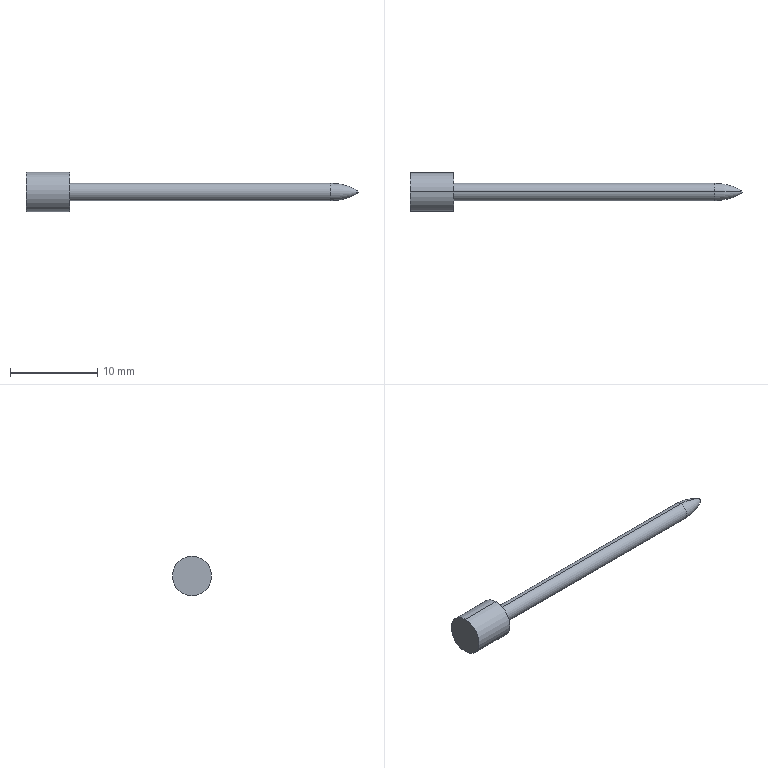Part | STEP file | BU-A09 | 1 solid | 10 faces | box 38.05 x 4.5 x 4.5 mm | volume 179.303 mm3 | cylinder 4 | plane 2 | other 2 | sphere 2 | commonest cylinder face diameters 2 x2 4.5 x2
STEP:
#1=CARTESIAN_POINT('',(0.,0.,0.));
#2=DIRECTION('',(0.,0.,1.));
#3=DIRECTION('',(1.,0.,0.));
#4=AXIS2_PLACEMENT_3D('',#1,#2,#3);
#5=CARTESIAN_POINT('',(5.,0.,2.25));
#6=VERTEX_POINT('',#5);
#7=CARTESIAN_POINT('',(5.,0.,-2.25));
#8=VERTEX_POINT('',#7);
#9=CARTESIAN_POINT('',(5.,0.,0.));
#10=DIRECTION('',(-1.,0.,0.));
#11=DIRECTION('',(0.,0.,1.));
#12=AXIS2_PLACEMENT_3D('',#9,#10,#11);
#13=CIRCLE('',#12,2.25);
#14=CARTESIAN_POINT('',(-1000.,0.,0.));
#15=DIRECTION('',(-1.,0.,0.));
#16=DIRECTION('',(0.,0.,1.));
#17=AXIS2_PLACEMENT_3D('',#14,#15,#16);
#18=CYLINDRICAL_SURFACE('',#17,2.25);
#19=CARTESIAN_POINT('',(0.,-1005.));
#20=DIRECTION('',(1.,0.));
#21=VECTOR('',#20,1.);
#22=LINE('',#19,#21);
#23=(GEOMETRIC_REPRESENTATION_CONTEXT(2)PARAMETRIC_REPRESENTATION_CONTEXT()REPRESENTATION_CONTEXT('',''));
#24=DEFINITIONAL_REPRESENTATION('',(#22),#23);
#25=PCURVE('',#18,#24);
#26=CARTESIAN_POINT('',(5.,2.25,0.));
#27=DIRECTION('',(-1.,0.,0.));
#28=DIRECTION('',(0.,0.,1.));
#29=AXIS2_PLACEMENT_3D('',#26,#27,#28);
#30=PLANE('',#29);
#31=CARTESIAN_POINT('',(0.,-2.25));
#32=DIRECTION('',(1.,0.));
#33=AXIS2_PLACEMENT_2D('',#31,#32);
#34=CIRCLE('',#33,2.25);
#35=(GEOMETRIC_REPRESENTATION_CONTEXT(2)PARAMETRIC_REPRESENTATION_CONTEXT()REPRESENTATION_CONTEXT('',''));
#36=DEFINITIONAL_REPRESENTATION('',(#34),#35);
#37=PCURVE('',#30,#36);
#38=SURFACE_CURVE('',#13,(#25,#37),.PCURVE_S1.);
#39=EDGE_CURVE('',#6,#8,#38,.T.);
#40=ORIENTED_EDGE('',*,*,#39,.T.);
#41=CARTESIAN_POINT('',(0.,0.,-2.25));
#42=VERTEX_POINT('',#41);
#43=CARTESIAN_POINT('',(-1000.,0.,-2.25));
#44=DIRECTION('',(-1.,0.,0.));
#45=VECTOR('',#44,1.);
#46=LINE('',#43,#45);
#47=CARTESIAN_POINT('',(3.142,0.));
#48=DIRECTION('',(0.,1.));
#49=VECTOR('',#48,1.);
#50=LINE('',#47,#49);
#51=(GEOMETRIC_REPRESENTATION_CONTEXT(2)PARAMETRIC_REPRESENTATION_CONTEXT()REPRESENTATION_CONTEXT('',''));
#52=DEFINITIONAL_REPRESENTATION('',(#50),#51);
#53=PCURVE('',#18,#52);
#54=CARTESIAN_POINT('',(-1000.,0.,0.));
#55=DIRECTION('',(-1.,0.,0.));
#56=DIRECTION('',(0.,0.,1.));
#57=AXIS2_PLACEMENT_3D('',#54,#55,#56);
#58=CYLINDRICAL_SURFACE('',#57,2.25);
#59=CARTESIAN_POINT('',(3.142,0.));
#60=DIRECTION('',(0.,1.));
#61=VECTOR('',#60,1.);
#62=LINE('',#59,#61);
#63=(GEOMETRIC_REPRESENTATION_CONTEXT(2)PARAMETRIC_REPRESENTATION_CONTEXT()REPRESENTATION_CONTEXT('',''));
#64=DEFINITIONAL_REPRESENTATION('',(#62),#63);
#65=PCURVE('',#58,#64);
#66=SURFACE_CURVE('',#46,(#53,#65),.PCURVE_S1.);
#67=EDGE_CURVE('',#8,#42,#66,.T.);
#68=ORIENTED_EDGE('',*,*,#67,.T.);
#69=CARTESIAN_POINT('',(0.,0.,2.25));
#70=VERTEX_POINT('',#69);
#71=CARTESIAN_POINT('',(0.,0.,0.));
#72=DIRECTION('',(-1.,0.,0.));
#73=DIRECTION('',(0.,0.,1.));
#74=AXIS2_PLACEMENT_3D('',#71,#72,#73);
#75=CIRCLE('',#74,2.25);
#76=CARTESIAN_POINT('',(0.,-1000.));
#77=DIRECTION('',(1.,0.));
#78=VECTOR('',#77,1.);
#79=LINE('',#76,#78);
#80=(GEOMETRIC_REPRESENTATION_CONTEXT(2)PARAMETRIC_REPRESENTATION_CONTEXT()REPRESENTATION_CONTEXT('',''));
#81=DEFINITIONAL_REPRESENTATION('',(#79),#80);
#82=PCURVE('',#18,#81);
#83=CARTESIAN_POINT('',(0.,0.,0.));
#84=DIRECTION('',(1.,0.,0.));
#85=DIRECTION('',(0.,0.,-1.));
#86=AXIS2_PLACEMENT_3D('',#83,#84,#85);
#87=PLANE('',#86);
#88=CARTESIAN_POINT('',(-2.25,0.));
#89=CARTESIAN_POINT('',(-2.25,3.897));
#90=CARTESIAN_POINT('',(1.125,1.949));
#91=CARTESIAN_POINT('',(4.5,0.));
#92=CARTESIAN_POINT('',(1.125,-1.949));
#93=CARTESIAN_POINT('',(-2.25,-3.897));
#94=CARTESIAN_POINT('',(-2.25,0.));
#95=(BOUNDED_CURVE()B_SPLINE_CURVE(2,(#88,#89,#90,#91,#92,#93,#94),.UNSPECIFIED.,.T.,.F.)B_SPLINE_CURVE_WITH_KNOTS((1,2,2,2,2,1),(-2.094,0.,2.094,4.189,6.283,8.378),.UNSPECIFIED.)CURVE()GEOMETRIC_REPRESENTATION_ITEM()RATIONAL_B_SPLINE_CURVE((1.,0.5,1.,0.5,1.,0.5,1.))REPRESENTATION_ITEM(''));
#96=(GEOMETRIC_REPRESENTATION_CONTEXT(2)PARAMETRIC_REPRESENTATION_CONTEXT()REPRESENTATION_CONTEXT('',''));
#97=DEFINITIONAL_REPRESENTATION('',(#95),#96);
#98=PCURVE('',#87,#97);
#99=SURFACE_CURVE('',#75,(#82,#98),.PCURVE_S1.);
#100=EDGE_CURVE('',#70,#42,#99,.T.);
#101=ORIENTED_EDGE('',*,*,#100,.F.);
#102=CARTESIAN_POINT('',(-1000.,0.,2.25));
#103=DIRECTION('',(-1.,0.,0.));
#104=VECTOR('',#103,1.);
#105=LINE('',#102,#104);
#106=CARTESIAN_POINT('',(0.,0.));
#107=DIRECTION('',(0.,1.));
#108=VECTOR('',#107,1.);
#109=LINE('',#106,#108);
#110=(GEOMETRIC_REPRESENTATION_CONTEXT(2)PARAMETRIC_REPRESENTATION_CONTEXT()REPRESENTATION_CONTEXT('',''));
#111=DEFINITIONAL_REPRESENTATION('',(#109),#110);
#112=PCURVE('',#18,#111);
#113=CARTESIAN_POINT('',(6.283,0.));
#114=DIRECTION('',(0.,1.));
#115=VECTOR('',#114,1.);
#116=LINE('',#113,#115);
#117=(GEOMETRIC_REPRESENTATION_CONTEXT(2)PARAMETRIC_REPRESENTATION_CONTEXT()REPRESENTATION_CONTEXT('',''));
#118=DEFINITIONAL_REPRESENTATION('',(#116),#117);
#119=PCURVE('',#58,#118);
#120=SURFACE_CURVE('',#105,(#112,#119),.PCURVE_S1.);
#121=EDGE_CURVE('',#6,#70,#120,.T.);
#122=ORIENTED_EDGE('',*,*,#121,.F.);
#123=EDGE_LOOP('',(#40,#68,#101,#122));
#124=FACE_BOUND('',#123,.T.);
#125=ADVANCED_FACE('',(#124),#18,.T.);
#126=ORIENTED_EDGE('',*,*,#100,.T.);
#127=CARTESIAN_POINT('',(0.,0.,0.));
#128=DIRECTION('',(-1.,0.,0.));
#129=DIRECTION('',(0.,0.,1.));
#130=AXIS2_PLACEMENT_3D('',#127,#128,#129);
#131=CIRCLE('',#130,2.25);
#132=CARTESIAN_POINT('',(-2.25,0.));
#133=CARTESIAN_POINT('',(-2.25,3.897));
#134=CARTESIAN_POINT('',(1.125,1.949));
#135=CARTESIAN_POINT('',(4.5,0.));
#136=CARTESIAN_POINT('',(1.125,-1.949));
#137=CARTESIAN_POINT('',(-2.25,-3.897));
#138=CARTESIAN_POINT('',(-2.25,0.));
#139=(BOUNDED_CURVE()B_SPLINE_CURVE(2,(#132,#133,#134,#135,#136,#137,#138),.UNSPECIFIED.,.T.,.F.)B_SPLINE_CURVE_WITH_KNOTS((1,2,2,2,2,1),(-2.094,0.,2.094,4.189,6.283,8.378),.UNSPECIFIED.)CURVE()GEOMETRIC_REPRESENTATION_ITEM()RATIONAL_B_SPLINE_CURVE((1.,0.5,1.,0.5,1.,0.5,1.))REPRESENTATION_ITEM(''));
#140=(GEOMETRIC_REPRESENTATION_CONTEXT(2)PARAMETRIC_REPRESENTATION_CONTEXT()REPRESENTATION_CONTEXT('',''));
#141=DEFINITIONAL_REPRESENTATION('',(#139),#140);
#142=PCURVE('',#87,#141);
#143=CARTESIAN_POINT('',(0.,-1000.));
#144=DIRECTION('',(1.,0.));
#145=VECTOR('',#144,1.);
#146=LINE('',#143,#145);
#147=(GEOMETRIC_REPRESENTATION_CONTEXT(2)PARAMETRIC_REPRESENTATION_CONTEXT()REPRESENTATION_CONTEXT('',''));
#148=DEFINITIONAL_REPRESENTATION('',(#146),#147);
#149=PCURVE('',#58,#148);
#150=SURFACE_CURVE('',#131,(#142,#149),.PCURVE_S1.);
#151=EDGE_CURVE('',#42,#70,#150,.T.);
#152=ORIENTED_EDGE('',*,*,#151,.T.);
#153=EDGE_LOOP('',(#126,#152));
#154=FACE_BOUND('',#153,.T.);
#155=ADVANCED_FACE('',(#154),#87,.F.);
#156=ORIENTED_EDGE('',*,*,#67,.F.);
#157=CARTESIAN_POINT('',(5.,0.,0.));
#158=DIRECTION('',(-1.,0.,0.));
#159=DIRECTION('',(0.,0.,1.));
#160=AXIS2_PLACEMENT_3D('',#157,#158,#159);
#161=CIRCLE('',#160,2.25);
#162=CARTESIAN_POINT('',(0.,-1005.));
#163=DIRECTION('',(1.,0.));
#164=VECTOR('',#163,1.);
#165=LINE('',#162,#164);
#166=(GEOMETRIC_REPRESENTATION_CONTEXT(2)PARAMETRIC_REPRESENTATION_CONTEXT()REPRESENTATION_CONTEXT('',''));
#167=DEFINITIONAL_REPRESENTATION('',(#165),#166);
#168=PCURVE('',#58,#167);
#169=CARTESIAN_POINT('',(0.,-2.25));
#170=DIRECTION('',(1.,0.));
#171=AXIS2_PLACEMENT_2D('',#169,#170);
#172=CIRCLE('',#171,2.25);
#173=(GEOMETRIC_REPRESENTATION_CONTEXT(2)PARAMETRIC_REPRESENTATION_CONTEXT()REPRESENTATION_CONTEXT('',''));
#174=DEFINITIONAL_REPRESENTATION('',(#172),#173);
#175=PCURVE('',#30,#174);
#176=SURFACE_CURVE('',#161,(#168,#175),.PCURVE_S1.);
#177=EDGE_CURVE('',#8,#6,#176,.T.);
#178=ORIENTED_EDGE('',*,*,#177,.T.);
#179=ORIENTED_EDGE('',*,*,#121,.T.);
#180=ORIENTED_EDGE('',*,*,#151,.F.);
#181=EDGE_LOOP('',(#156,#178,#179,#180));
#182=FACE_BOUND('',#181,.T.);
#183=ADVANCED_FACE('',(#182),#58,.T.);
#184=ORIENTED_EDGE('',*,*,#39,.F.);
#185=ORIENTED_EDGE('',*,*,#177,.F.);
#186=EDGE_LOOP('',(#184,#185));
#187=FACE_BOUND('',#186,.T.);
#188=CARTESIAN_POINT('',(5.,0.,1.));
#189=VERTEX_POINT('',#188);
#190=CARTESIAN_POINT('',(5.,0.,-1.));
#191=VERTEX_POINT('',#190);
#192=CARTESIAN_POINT('',(5.,0.,0.));
#193=DIRECTION('',(-1.,0.,0.));
#194=DIRECTION('',(0.,0.,1.));
#195=AXIS2_PLACEMENT_3D('',#192,#193,#194);
#196=CIRCLE('',#195,1.);
#197=CARTESIAN_POINT('',(0.,-2.25));
#198=DIRECTION('',(1.,0.));
#199=AXIS2_PLACEMENT_2D('',#197,#198);
#200=CIRCLE('',#199,1.);
#201=(GEOMETRIC_REPRESENTATION_CONTEXT(2)PARAMETRIC_REPRESENTATION_CONTEXT()REPRESENTATION_CONTEXT('',''));
#202=DEFINITIONAL_REPRESENTATION('',(#200),#201);
#203=PCURVE('',#30,#202);
#204=CARTESIAN_POINT('',(-1000.,0.,0.));
#205=DIRECTION('',(-1.,0.,0.));
#206=DIRECTION('',(0.,0.,1.));
#207=AXIS2_PLACEMENT_3D('',#204,#205,#206);
#208=CYLINDRICAL_SURFACE('',#207,1.);
#209=CARTESIAN_POINT('',(0.,-1005.));
#210=DIRECTION('',(1.,0.));
#211=VECTOR('',#210,1.);
#212=LINE('',#209,#211);
#213=(GEOMETRIC_REPRESENTATION_CONTEXT(2)PARAMETRIC_REPRESENTATION_CONTEXT()REPRESENTATION_CONTEXT('',''));
#214=DEFINITIONAL_REPRESENTATION('',(#212),#213);
#215=PCURVE('',#208,#214);
#216=SURFACE_CURVE('',#196,(#203,#215),.PCURVE_S1.);
#217=EDGE_CURVE('',#189,#191,#216,.T.);
#218=ORIENTED_EDGE('',*,*,#217,.T.);
#219=CARTESIAN_POINT('',(5.,0.,0.));
#220=DIRECTION('',(-1.,0.,0.));
#221=DIRECTION('',(0.,0.,1.));
#222=AXIS2_PLACEMENT_3D('',#219,#220,#221);
#223=CIRCLE('',#222,1.);
#224=CARTESIAN_POINT('',(0.,-2.25));
#225=DIRECTION('',(1.,0.));
#226=AXIS2_PLACEMENT_2D('',#224,#225);
#227=CIRCLE('',#226,1.);
#228=(GEOMETRIC_REPRESENTATION_CONTEXT(2)PARAMETRIC_REPRESENTATION_CONTEXT()REPRESENTATION_CONTEXT('',''));
#229=DEFINITIONAL_REPRESENTATION('',(#227),#228);
#230=PCURVE('',#30,#229);
#231=CARTESIAN_POINT('',(-1000.,0.,0.));
#232=DIRECTION('',(-1.,0.,0.));
#233=DIRECTION('',(0.,0.,1.));
#234=AXIS2_PLACEMENT_3D('',#231,#232,#233);
#235=CYLINDRICAL_SURFACE('',#234,1.);
#236=CARTESIAN_POINT('',(0.,-1005.));
#237=DIRECTION('',(1.,0.));
#238=VECTOR('',#237,1.);
#239=LINE('',#236,#238);
#240=(GEOMETRIC_REPRESENTATION_CONTEXT(2)PARAMETRIC_REPRESENTATION_CONTEXT()REPRESENTATION_CONTEXT('',''));
#241=DEFINITIONAL_REPRESENTATION('',(#239),#240);
#242=PCURVE('',#235,#241);
#243=SURFACE_CURVE('',#223,(#230,#242),.PCURVE_S1.);
#244=EDGE_CURVE('',#191,#189,#243,.T.);
#245=ORIENTED_EDGE('',*,*,#244,.T.);
#246=EDGE_LOOP('',(#218,#245));
#247=FACE_BOUND('',#246,.T.);
#248=ADVANCED_FACE('',(#187,#247),#30,.F.);
#249=CARTESIAN_POINT('',(34.934,0.,-1.));
#250=VERTEX_POINT('',#249);
#251=CARTESIAN_POINT('',(-1000.,0.,-1.));
#252=DIRECTION('',(-1.,0.,0.));
#253=VECTOR('',#252,1.);
#254=LINE('',#251,#253);
#255=CARTESIAN_POINT('',(3.142,0.));
#256=DIRECTION('',(0.,1.));
#257=VECTOR('',#256,1.);
#258=LINE('',#255,#257);
#259=(GEOMETRIC_REPRESENTATION_CONTEXT(2)PARAMETRIC_REPRESENTATION_CONTEXT()REPRESENTATION_CONTEXT('',''));
#260=DEFINITIONAL_REPRESENTATION('',(#258),#259);
#261=PCURVE('',#235,#260);
#262=CARTESIAN_POINT('',(3.142,0.));
#263=DIRECTION('',(0.,1.));
#264=VECTOR('',#263,1.);
#265=LINE('',#262,#264);
#266=(GEOMETRIC_REPRESENTATION_CONTEXT(2)PARAMETRIC_REPRESENTATION_CONTEXT()REPRESENTATION_CONTEXT('',''));
#267=DEFINITIONAL_REPRESENTATION('',(#265),#266);
#268=PCURVE('',#208,#267);
#269=SURFACE_CURVE('',#254,(#261,#268),.PCURVE_S1.);
#270=EDGE_CURVE('',#250,#191,#269,.T.);
#271=ORIENTED_EDGE('',*,*,#270,.F.);
#272=CARTESIAN_POINT('',(34.934,0.,1.));
#273=VERTEX_POINT('',#272);
#274=CARTESIAN_POINT('',(34.934,0.,0.));
#275=DIRECTION('',(-1.,0.,0.));
#276=DIRECTION('',(0.,0.,1.));
#277=AXIS2_PLACEMENT_3D('',#274,#275,#276);
#278=CIRCLE('',#277,1.);
#279=CARTESIAN_POINT('',(0.,-1034.934));
#280=DIRECTION('',(1.,0.));
#281=VECTOR('',#280,1.);
#282=LINE('',#279,#281);
#283=(GEOMETRIC_REPRESENTATION_CONTEXT(2)PARAMETRIC_REPRESENTATION_CONTEXT()REPRESENTATION_CONTEXT('',''));
#284=DEFINITIONAL_REPRESENTATION('',(#282),#283);
#285=PCURVE('',#235,#284);
#286=CARTESIAN_POINT('',(34.934,0.,-1.));
#287=CARTESIAN_POINT('',(35.559,0.,-1.));
#288=CARTESIAN_POINT('',(36.183,0.,-0.9201));
#289=CARTESIAN_POINT('',(36.794,0.,-0.7602));
#290=CARTESIAN_POINT('',(37.378,0.,-0.5239));
#291=CARTESIAN_POINT('',(37.922,0.,-0.2179));
#292=B_SPLINE_CURVE_WITH_KNOTS('',5,(#286,#287,#288,#289,#290,#291),.UNSPECIFIED.,.F.,.F.,(6,6),(3.142,3.654),.PIECEWISE_BEZIER_KNOTS.);
#293=CARTESIAN_POINT('',(34.934,0.,0.));
#294=DIRECTION('',(-1.,0.,0.));
#295=AXIS1_PLACEMENT('',#293,#294);
#296=SURFACE_OF_REVOLUTION('',#292,#295);
#297=CARTESIAN_POINT('',(-3.142,3.142));
#298=DIRECTION('',(1.,0.));
#299=VECTOR('',#298,1.);
#300=LINE('',#297,#299);
#301=(GEOMETRIC_REPRESENTATION_CONTEXT(2)PARAMETRIC_REPRESENTATION_CONTEXT()REPRESENTATION_CONTEXT('',''));
#302=DEFINITIONAL_REPRESENTATION('',(#300),#301);
#303=PCURVE('',#296,#302);
#304=SURFACE_CURVE('',#278,(#285,#303),.PCURVE_S1.);
#305=EDGE_CURVE('',#250,#273,#304,.T.);
#306=ORIENTED_EDGE('',*,*,#305,.T.);
#307=CARTESIAN_POINT('',(-1000.,0.,1.));
#308=DIRECTION('',(-1.,0.,0.));
#309=VECTOR('',#308,1.);
#310=LINE('',#307,#309);
#311=CARTESIAN_POINT('',(6.283,0.));
#312=DIRECTION('',(0.,1.));
#313=VECTOR('',#312,1.);
#314=LINE('',#311,#313);
#315=(GEOMETRIC_REPRESENTATION_CONTEXT(2)PARAMETRIC_REPRESENTATION_CONTEXT()REPRESENTATION_CONTEXT('',''));
#316=DEFINITIONAL_REPRESENTATION('',(#314),#315);
#317=PCURVE('',#235,#316);
#318=CARTESIAN_POINT('',(0.,0.));
#319=DIRECTION('',(0.,1.));
#320=VECTOR('',#319,1.);
#321=LINE('',#318,#320);
#322=(GEOMETRIC_REPRESENTATION_CONTEXT(2)PARAMETRIC_REPRESENTATION_CONTEXT()REPRESENTATION_CONTEXT('',''));
#323=DEFINITIONAL_REPRESENTATION('',(#321),#322);
#324=PCURVE('',#208,#323);
#325=SURFACE_CURVE('',#310,(#317,#324),.PCURVE_S1.);
#326=EDGE_CURVE('',#273,#189,#325,.T.);
#327=ORIENTED_EDGE('',*,*,#326,.T.);
#328=ORIENTED_EDGE('',*,*,#244,.F.);
#329=EDGE_LOOP('',(#271,#306,#327,#328));
#330=FACE_BOUND('',#329,.T.);
#331=ADVANCED_FACE('',(#330),#235,.T.);
#332=ORIENTED_EDGE('',*,*,#305,.T.);
#333=CARTESIAN_POINT('',(37.922,0.,0.2179));
#334=VERTEX_POINT('',#333);
#335=CARTESIAN_POINT('',(34.934,0.,-5.1));
#336=DIRECTION('',(0.,-1.,0.));
#337=DIRECTION('',(1.,0.,0.));
#338=AXIS2_PLACEMENT_3D('',#335,#336,#337);
#339=CIRCLE('',#338,6.1);
#340=CARTESIAN_POINT('',(3.142,4.712));
#341=DIRECTION('',(0.,-1.));
#342=VECTOR('',#341,1.);
#343=LINE('',#340,#342);
#344=(GEOMETRIC_REPRESENTATION_CONTEXT(2)PARAMETRIC_REPRESENTATION_CONTEXT()REPRESENTATION_CONTEXT('',''));
#345=DEFINITIONAL_REPRESENTATION('',(#343),#344);
#346=PCURVE('',#296,#345);
#347=CARTESIAN_POINT('',(34.934,0.,-1.));
#348=CARTESIAN_POINT('',(35.559,0.,-1.));
#349=CARTESIAN_POINT('',(36.183,0.,-0.9201));
#350=CARTESIAN_POINT('',(36.794,0.,-0.7602));
#351=CARTESIAN_POINT('',(37.378,0.,-0.5239));
#352=CARTESIAN_POINT('',(37.922,0.,-0.2179));
#353=B_SPLINE_CURVE_WITH_KNOTS('',5,(#347,#348,#349,#350,#351,#352),.UNSPECIFIED.,.F.,.F.,(6,6),(3.142,3.654),.PIECEWISE_BEZIER_KNOTS.);
#354=CARTESIAN_POINT('',(34.934,0.,0.));
#355=DIRECTION('',(-1.,0.,0.));
#356=AXIS1_PLACEMENT('',#354,#355);
#357=SURFACE_OF_REVOLUTION('',#353,#356);
#358=CARTESIAN_POINT('',(3.142,4.712));
#359=DIRECTION('',(0.,-1.));
#360=VECTOR('',#359,1.);
#361=LINE('',#358,#360);
#362=(GEOMETRIC_REPRESENTATION_CONTEXT(2)PARAMETRIC_REPRESENTATION_CONTEXT()REPRESENTATION_CONTEXT('',''));
#363=DEFINITIONAL_REPRESENTATION('',(#361),#362);
#364=PCURVE('',#357,#363);
#365=SURFACE_CURVE('',#339,(#346,#364),.PCURVE_S1.);
#366=EDGE_CURVE('',#334,#273,#365,.T.);
#367=ORIENTED_EDGE('',*,*,#366,.F.);
#368=CARTESIAN_POINT('',(37.922,-0.2179,0.));
#369=VERTEX_POINT('',#368);
#370=CARTESIAN_POINT('',(37.922,0.,0.));
#371=DIRECTION('',(-1.,0.,0.));
#372=DIRECTION('',(0.,0.,1.));
#373=AXIS2_PLACEMENT_3D('',#370,#371,#372);
#374=CIRCLE('',#373,0.2179);
#375=CARTESIAN_POINT('',(-3.142,3.654));
#376=DIRECTION('',(1.,0.));
#377=VECTOR('',#376,1.);
#378=LINE('',#375,#377);
#379=(GEOMETRIC_REPRESENTATION_CONTEXT(2)PARAMETRIC_REPRESENTATION_CONTEXT()REPRESENTATION_CONTEXT('',''));
#380=DEFINITIONAL_REPRESENTATION('',(#378),#379);
#381=PCURVE('',#296,#380);
#382=CARTESIAN_POINT('',(37.8,0.,0.));
#383=DIRECTION('',(0.,0.,-1.));
#384=DIRECTION('',(0.,1.,0.));
#385=AXIS2_PLACEMENT_3D('',#382,#383,#384);
#386=SPHERICAL_SURFACE('',#385,0.25);
#387=CARTESIAN_POINT('',(2.63,0.));
#388=CARTESIAN_POINT('',(2.63,-0.02075));
#389=CARTESIAN_POINT('',(2.629,-0.06225));
#390=CARTESIAN_POINT('',(2.626,-0.1244));
#391=CARTESIAN_POINT('',(2.62,-0.1864));
#392=CARTESIAN_POINT('',(2.612,-0.2482));
#393=CARTESIAN_POINT('',(2.602,-0.3097));
#394=CARTESIAN_POINT('',(2.589,-0.3707));
#395=CARTESIAN_POINT('',(2.573,-0.4311));
#396=CARTESIAN_POINT('',(2.553,-0.4909));
#397=CARTESIAN_POINT('',(2.53,-0.5499));
#398=CARTESIAN_POINT('',(2.503,-0.6078));
#399=CARTESIAN_POINT('',(2.471,-0.6645));
#400=CARTESIAN_POINT('',(2.433,-0.7196));
#401=CARTESIAN_POINT('',(2.39,-0.7729));
#402=CARTESIAN_POINT('',(2.338,-0.8238));
#403=CARTESIAN_POINT('',(2.279,-0.8719));
#404=CARTESIAN_POINT('',(2.209,-0.9165));
#405=CARTESIAN_POINT('',(2.129,-0.9568));
#406=CARTESIAN_POINT('',(2.037,-0.9919));
#407=CARTESIAN_POINT('',(1.934,-1.021));
#408=CARTESIAN_POINT('',(1.82,-1.042));
#409=CARTESIAN_POINT('',(1.698,-1.056));
#410=CARTESIAN_POINT('',(1.613,-1.059));
#411=CARTESIAN_POINT('',(1.571,-1.059));
#412=B_SPLINE_CURVE_WITH_KNOTS('',3,(#387,#388,#389,#390,#391,#392,#393,#394,#395,#396,#397,#398,#399,#400,#401,#402,#403,#404,#405,#406,#407,#408,#409,#410,#411),.UNSPECIFIED.,.F.,.F.,(4,1,1,1,1,1,1,1,1,1,1,1,1,1,1,1,1,1,1,1,1,1,4),(4.712,4.784,4.855,4.927,4.998,5.069,5.141,5.212,5.284,5.355,5.426,5.498,5.569,5.641,5.712,5.783,5.855,5.926,5.998,6.069,6.14,6.212,6.283),.QUASI_UNIFORM_KNOTS.);
#413=(GEOMETRIC_REPRESENTATION_CONTEXT(2)PARAMETRIC_REPRESENTATION_CONTEXT()REPRESENTATION_CONTEXT('',''));
#414=DEFINITIONAL_REPRESENTATION('',(#412),#413);
#415=PCURVE('',#386,#414);
#416=SURFACE_CURVE('',#374,(#381,#415),.PCURVE_S1.);
#417=EDGE_CURVE('',#369,#334,#416,.T.);
#418=ORIENTED_EDGE('',*,*,#417,.F.);
#419=CARTESIAN_POINT('',(37.922,0.,-0.2179));
#420=VERTEX_POINT('',#419);
#421=CARTESIAN_POINT('',(37.922,0.,0.));
#422=DIRECTION('',(-1.,0.,0.));
#423=DIRECTION('',(0.,0.,1.));
#424=AXIS2_PLACEMENT_3D('',#421,#422,#423);
#425=CIRCLE('',#424,0.2179);
#426=CARTESIAN_POINT('',(-3.142,3.654));
#427=DIRECTION('',(1.,0.));
#428=VECTOR('',#427,1.);
#429=LINE('',#426,#428);
#430=(GEOMETRIC_REPRESENTATION_CONTEXT(2)PARAMETRIC_REPRESENTATION_CONTEXT()REPRESENTATION_CONTEXT('',''));
#431=DEFINITIONAL_REPRESENTATION('',(#429),#430);
#432=PCURVE('',#296,#431);
#433=CARTESIAN_POINT('',(37.8,0.,0.));
#434=DIRECTION('',(0.,0.,-1.));
#435=DIRECTION('',(0.,1.,0.));
#436=AXIS2_PLACEMENT_3D('',#433,#434,#435);
#437=SPHERICAL_SURFACE('',#436,0.25);
#438=CARTESIAN_POINT('',(1.571,1.059));
#439=CARTESIAN_POINT('',(1.613,1.059));
#440=CARTESIAN_POINT('',(1.698,1.056));
#441=CARTESIAN_POINT('',(1.82,1.042));
#442=CARTESIAN_POINT('',(1.934,1.021));
#443=CARTESIAN_POINT('',(2.037,0.9919));
#444=CARTESIAN_POINT('',(2.129,0.9568));
#445=CARTESIAN_POINT('',(2.209,0.9165));
#446=CARTESIAN_POINT('',(2.279,0.8719));
#447=CARTESIAN_POINT('',(2.338,0.8238));
#448=CARTESIAN_POINT('',(2.39,0.7729));
#449=CARTESIAN_POINT('',(2.433,0.7196));
#450=CARTESIAN_POINT('',(2.471,0.6645));
#451=CARTESIAN_POINT('',(2.503,0.6078));
#452=CARTESIAN_POINT('',(2.53,0.5499));
#453=CARTESIAN_POINT('',(2.553,0.4909));
#454=CARTESIAN_POINT('',(2.573,0.4311));
#455=CARTESIAN_POINT('',(2.589,0.3707));
#456=CARTESIAN_POINT('',(2.602,0.3097));
#457=CARTESIAN_POINT('',(2.612,0.2482));
#458=CARTESIAN_POINT('',(2.62,0.1864));
#459=CARTESIAN_POINT('',(2.626,0.1244));
#460=CARTESIAN_POINT('',(2.629,0.06225));
#461=CARTESIAN_POINT('',(2.63,0.02075));
#462=CARTESIAN_POINT('',(2.63,0.));
#463=B_SPLINE_CURVE_WITH_KNOTS('',3,(#438,#439,#440,#441,#442,#443,#444,#445,#446,#447,#448,#449,#450,#451,#452,#453,#454,#455,#456,#457,#458,#459,#460,#461,#462),.UNSPECIFIED.,.F.,.F.,(4,1,1,1,1,1,1,1,1,1,1,1,1,1,1,1,1,1,1,1,1,1,4),(3.142,3.213,3.284,3.356,3.427,3.499,3.57,3.641,3.713,3.784,3.856,3.927,3.998,4.07,4.141,4.213,4.284,4.355,4.427,4.498,4.57,4.641,4.712),.QUASI_UNIFORM_KNOTS.);
#464=(GEOMETRIC_REPRESENTATION_CONTEXT(2)PARAMETRIC_REPRESENTATION_CONTEXT()REPRESENTATION_CONTEXT('',''));
#465=DEFINITIONAL_REPRESENTATION('',(#463),#464);
#466=PCURVE('',#437,#465);
#467=SURFACE_CURVE('',#425,(#432,#466),.PCURVE_S1.);
#468=EDGE_CURVE('',#420,#369,#467,.T.);
#469=ORIENTED_EDGE('',*,*,#468,.F.);
#470=CARTESIAN_POINT('',(34.934,0.,5.1));
#471=DIRECTION('',(0.,1.,0.));
#472=DIRECTION('',(0.,0.,1.));
#473=AXIS2_PLACEMENT_3D('',#470,#471,#472);
#474=CIRCLE('',#473,6.1);
#475=CARTESIAN_POINT('',(0.,6.283));
#476=DIRECTION('',(0.,-1.));
#477=VECTOR('',#476,1.);
#478=LINE('',#475,#477);
#479=(GEOMETRIC_REPRESENTATION_CONTEXT(2)PARAMETRIC_REPRESENTATION_CONTEXT()REPRESENTATION_CONTEXT('',''));
#480=DEFINITIONAL_REPRESENTATION('',(#478),#479);
#481=PCURVE('',#296,#480);
#482=CARTESIAN_POINT('',(6.283,6.283));
#483=DIRECTION('',(0.,-1.));
#484=VECTOR('',#483,1.);
#485=LINE('',#482,#484);
#486=(GEOMETRIC_REPRESENTATION_CONTEXT(2)PARAMETRIC_REPRESENTATION_CONTEXT()REPRESENTATION_CONTEXT('',''));
#487=DEFINITIONAL_REPRESENTATION('',(#485),#486);
#488=PCURVE('',#357,#487);
#489=SURFACE_CURVE('',#474,(#481,#488),.PCURVE_S1.);
#490=EDGE_CURVE('',#420,#250,#489,.T.);
#491=ORIENTED_EDGE('',*,*,#490,.T.);
#492=EDGE_LOOP('',(#332,#367,#418,#469,#491));
#493=FACE_BOUND('',#492,.F.);
#494=ADVANCED_FACE('',(#493),#296,.F.);
#495=CARTESIAN_POINT('',(38.05,0.,0.));
#496=VERTEX_POINT('',#495);
#497=CARTESIAN_POINT('',(37.922,0.2179,0.));
#498=VERTEX_POINT('',#497);
#499=CARTESIAN_POINT('',(37.8,0.,0.));
#500=DIRECTION('',(0.,0.,1.));
#501=DIRECTION('',(1.,0.,0.));
#502=AXIS2_PLACEMENT_3D('',#499,#500,#501);
#503=CIRCLE('',#502,0.25);
#504=CARTESIAN_POINT('',(1.571,0.));
#505=DIRECTION('',(-1.,0.));
#506=VECTOR('',#505,1.);
#507=LINE('',#504,#506);
#508=(GEOMETRIC_REPRESENTATION_CONTEXT(2)PARAMETRIC_REPRESENTATION_CONTEXT()REPRESENTATION_CONTEXT('',''));
#509=DEFINITIONAL_REPRESENTATION('',(#507),#508);
#510=PCURVE('',#437,#509);
#511=CARTESIAN_POINT('',(1.571,0.));
#512=DIRECTION('',(-1.,0.));
#513=VECTOR('',#512,1.);
#514=LINE('',#511,#513);
#515=(GEOMETRIC_REPRESENTATION_CONTEXT(2)PARAMETRIC_REPRESENTATION_CONTEXT()REPRESENTATION_CONTEXT('',''));
#516=DEFINITIONAL_REPRESENTATION('',(#514),#515);
#517=PCURVE('',#386,#516);
#518=SURFACE_CURVE('',#503,(#510,#517),.PCURVE_S1.);
#519=EDGE_CURVE('',#496,#498,#518,.T.);
#520=ORIENTED_EDGE('',*,*,#519,.F.);
#521=CARTESIAN_POINT('',(37.8,0.,0.));
#522=DIRECTION('',(0.,0.,-1.));
#523=DIRECTION('',(0.,1.,0.));
#524=AXIS2_PLACEMENT_3D('',#521,#522,#523);
#525=CIRCLE('',#524,0.25);
#526=CARTESIAN_POINT('',(0.,0.));
#527=DIRECTION('',(1.,0.));
#528=VECTOR('',#527,1.);
#529=LINE('',#526,#528);
#530=(GEOMETRIC_REPRESENTATION_CONTEXT(2)PARAMETRIC_REPRESENTATION_CONTEXT()REPRESENTATION_CONTEXT('',''));
#531=DEFINITIONAL_REPRESENTATION('',(#529),#530);
#532=PCURVE('',#437,#531);
#533=CARTESIAN_POINT('',(0.,0.));
#534=DIRECTION('',(1.,0.));
#535=VECTOR('',#534,1.);
#536=LINE('',#533,#535);
#537=(GEOMETRIC_REPRESENTATION_CONTEXT(2)PARAMETRIC_REPRESENTATION_CONTEXT()REPRESENTATION_CONTEXT('',''));
#538=DEFINITIONAL_REPRESENTATION('',(#536),#537);
#539=PCURVE('',#386,#538);
#540=SURFACE_CURVE('',#525,(#532,#539),.PCURVE_S1.);
#541=EDGE_CURVE('',#496,#369,#540,.T.);
#542=ORIENTED_EDGE('',*,*,#541,.T.);
#543=ORIENTED_EDGE('',*,*,#468,.F.);
#544=CARTESIAN_POINT('',(37.922,0.,0.));
#545=DIRECTION('',(-1.,0.,0.));
#546=DIRECTION('',(0.,0.,1.));
#547=AXIS2_PLACEMENT_3D('',#544,#545,#546);
#548=CIRCLE('',#547,0.2179);
#549=CARTESIAN_POINT('',(0.5119,0.));
#550=CARTESIAN_POINT('',(0.5119,0.02075));
#551=CARTESIAN_POINT('',(0.5127,0.06225));
#552=CARTESIAN_POINT('',(0.5159,0.1244));
#553=CARTESIAN_POINT('',(0.5215,0.1864));
#554=CARTESIAN_POINT('',(0.5294,0.2482));
#555=CARTESIAN_POINT('',(0.5398,0.3097));
#556=CARTESIAN_POINT('',(0.5529,0.3707));
#557=CARTESIAN_POINT('',(0.5689,0.4311));
#558=CARTESIAN_POINT('',(0.5883,0.4909));
#559=CARTESIAN_POINT('',(0.6113,0.5499));
#560=CARTESIAN_POINT('',(0.6385,0.6078));
#561=CARTESIAN_POINT('',(0.6706,0.6645));
#562=CARTESIAN_POINT('',(0.7081,0.7196));
#563=CARTESIAN_POINT('',(0.752,0.7729));
#564=CARTESIAN_POINT('',(0.8033,0.8238));
#565=CARTESIAN_POINT('',(0.863,0.8719));
#566=CARTESIAN_POINT('',(0.9324,0.9165));
#567=CARTESIAN_POINT('',(1.012,0.9568));
#568=CARTESIAN_POINT('',(1.104,0.9919));
#569=CARTESIAN_POINT('',(1.207,1.021));
#570=CARTESIAN_POINT('',(1.321,1.042));
#571=CARTESIAN_POINT('',(1.444,1.056));
#572=CARTESIAN_POINT('',(1.528,1.059));
#573=CARTESIAN_POINT('',(1.571,1.059));
#574=B_SPLINE_CURVE_WITH_KNOTS('',3,(#549,#550,#551,#552,#553,#554,#555,#556,#557,#558,#559,#560,#561,#562,#563,#564,#565,#566,#567,#568,#569,#570,#571,#572,#573),.UNSPECIFIED.,.F.,.F.,(4,1,1,1,1,1,1,1,1,1,1,1,1,1,1,1,1,1,1,1,1,1,4),(1.571,1.642,1.714,1.785,1.856,1.928,1.999,2.071,2.142,2.213,2.285,2.356,2.428,2.499,2.57,2.642,2.713,2.785,2.856,2.927,2.999,3.07,3.142),.QUASI_UNIFORM_KNOTS.);
#575=(GEOMETRIC_REPRESENTATION_CONTEXT(2)PARAMETRIC_REPRESENTATION_CONTEXT()REPRESENTATION_CONTEXT('',''));
#576=DEFINITIONAL_REPRESENTATION('',(#574),#575);
#577=PCURVE('',#437,#576);
#578=CARTESIAN_POINT('',(3.142,3.654));
#579=DIRECTION('',(1.,0.));
#580=VECTOR('',#579,1.);
#581=LINE('',#578,#580);
#582=(GEOMETRIC_REPRESENTATION_CONTEXT(2)PARAMETRIC_REPRESENTATION_CONTEXT()REPRESENTATION_CONTEXT('',''));
#583=DEFINITIONAL_REPRESENTATION('',(#581),#582);
#584=PCURVE('',#357,#583);
#585=SURFACE_CURVE('',#548,(#577,#584),.PCURVE_S1.);
#586=EDGE_CURVE('',#498,#420,#585,.T.);
#587=ORIENTED_EDGE('',*,*,#586,.F.);
#588=EDGE_LOOP('',(#520,#542,#543,#587));
#589=FACE_BOUND('',#588,.T.);
#590=ADVANCED_FACE('',(#589),#437,.T.);
#591=ORIENTED_EDGE('',*,*,#541,.F.);
#592=ORIENTED_EDGE('',*,*,#519,.T.);
#593=CARTESIAN_POINT('',(37.922,0.,0.));
#594=DIRECTION('',(-1.,0.,0.));
#595=DIRECTION('',(0.,0.,1.));
#596=AXIS2_PLACEMENT_3D('',#593,#594,#595);
#597=CIRCLE('',#596,0.2179);
#598=CARTESIAN_POINT('',(1.571,-1.059));
#599=CARTESIAN_POINT('',(1.528,-1.059));
#600=CARTESIAN_POINT('',(1.444,-1.056));
#601=CARTESIAN_POINT('',(1.321,-1.042));
#602=CARTESIAN_POINT('',(1.207,-1.021));
#603=CARTESIAN_POINT('',(1.104,-0.9919));
#604=CARTESIAN_POINT('',(1.012,-0.9568));
#605=CARTESIAN_POINT('',(0.9324,-0.9165));
#606=CARTESIAN_POINT('',(0.863,-0.8719));
#607=CARTESIAN_POINT('',(0.8033,-0.8238));
#608=CARTESIAN_POINT('',(0.752,-0.7729));
#609=CARTESIAN_POINT('',(0.7081,-0.7196));
#610=CARTESIAN_POINT('',(0.6706,-0.6645));
#611=CARTESIAN_POINT('',(0.6385,-0.6078));
#612=CARTESIAN_POINT('',(0.6113,-0.5499));
#613=CARTESIAN_POINT('',(0.5883,-0.4909));
#614=CARTESIAN_POINT('',(0.5689,-0.4311));
#615=CARTESIAN_POINT('',(0.5529,-0.3707));
#616=CARTESIAN_POINT('',(0.5398,-0.3097));
#617=CARTESIAN_POINT('',(0.5294,-0.2482));
#618=CARTESIAN_POINT('',(0.5215,-0.1864));
#619=CARTESIAN_POINT('',(0.5159,-0.1244));
#620=CARTESIAN_POINT('',(0.5127,-0.06225));
#621=CARTESIAN_POINT('',(0.5119,-0.02075));
#622=CARTESIAN_POINT('',(0.5119,0.));
#623=B_SPLINE_CURVE_WITH_KNOTS('',3,(#598,#599,#600,#601,#602,#603,#604,#605,#606,#607,#608,#609,#610,#611,#612,#613,#614,#615,#616,#617,#618,#619,#620,#621,#622),.UNSPECIFIED.,.F.,.F.,(4,1,1,1,1,1,1,1,1,1,1,1,1,1,1,1,1,1,1,1,1,1,4),(0.,0.0714,0.1428,0.2142,0.2856,0.357,0.4284,0.4998,0.5712,0.6426,0.714,0.7854,0.8568,0.9282,0.9996,1.071,1.142,1.214,1.285,1.357,1.428,1.499,1.571),.QUASI_UNIFORM_KNOTS.);
#624=(GEOMETRIC_REPRESENTATION_CONTEXT(2)PARAMETRIC_REPRESENTATION_CONTEXT()REPRESENTATION_CONTEXT('',''));
#625=DEFINITIONAL_REPRESENTATION('',(#623),#624);
#626=PCURVE('',#386,#625);
#627=CARTESIAN_POINT('',(3.142,3.654));
#628=DIRECTION('',(1.,0.));
#629=VECTOR('',#628,1.);
#630=LINE('',#627,#629);
#631=(GEOMETRIC_REPRESENTATION_CONTEXT(2)PARAMETRIC_REPRESENTATION_CONTEXT()REPRESENTATION_CONTEXT('',''));
#632=DEFINITIONAL_REPRESENTATION('',(#630),#631);
#633=PCURVE('',#357,#632);
#634=SURFACE_CURVE('',#597,(#626,#633),.PCURVE_S1.);
#635=EDGE_CURVE('',#334,#498,#634,.T.);
#636=ORIENTED_EDGE('',*,*,#635,.F.);
#637=ORIENTED_EDGE('',*,*,#417,.F.);
#638=EDGE_LOOP('',(#591,#592,#636,#637));
#639=FACE_BOUND('',#638,.T.);
#640=ADVANCED_FACE('',(#639),#386,.T.);
#641=ORIENTED_EDGE('',*,*,#635,.F.);
#642=ORIENTED_EDGE('',*,*,#366,.T.);
#643=CARTESIAN_POINT('',(34.934,0.,0.));
#644=DIRECTION('',(-1.,0.,0.));
#645=DIRECTION('',(0.,0.,1.));
#646=AXIS2_PLACEMENT_3D('',#643,#644,#645);
#647=CIRCLE('',#646,1.);
#648=CARTESIAN_POINT('',(3.142,3.142));
#649=DIRECTION('',(1.,0.));
#650=VECTOR('',#649,1.);
#651=LINE('',#648,#650);
#652=(GEOMETRIC_REPRESENTATION_CONTEXT(2)PARAMETRIC_REPRESENTATION_CONTEXT()REPRESENTATION_CONTEXT('',''));
#653=DEFINITIONAL_REPRESENTATION('',(#651),#652);
#654=PCURVE('',#357,#653);
#655=CARTESIAN_POINT('',(0.,-1034.934));
#656=DIRECTION('',(1.,0.));
#657=VECTOR('',#656,1.);
#658=LINE('',#655,#657);
#659=(GEOMETRIC_REPRESENTATION_CONTEXT(2)PARAMETRIC_REPRESENTATION_CONTEXT()REPRESENTATION_CONTEXT('',''));
#660=DEFINITIONAL_REPRESENTATION('',(#658),#659);
#661=PCURVE('',#208,#660);
#662=SURFACE_CURVE('',#647,(#654,#661),.PCURVE_S1.);
#663=EDGE_CURVE('',#273,#250,#662,.T.);
#664=ORIENTED_EDGE('',*,*,#663,.T.);
#665=ORIENTED_EDGE('',*,*,#490,.F.);
#666=ORIENTED_EDGE('',*,*,#586,.F.);
#667=EDGE_LOOP('',(#641,#642,#664,#665,#666));
#668=FACE_BOUND('',#667,.F.);
#669=ADVANCED_FACE('',(#668),#357,.F.);
#670=ORIENTED_EDGE('',*,*,#663,.T.);
#671=ORIENTED_EDGE('',*,*,#270,.T.);
#672=ORIENTED_EDGE('',*,*,#217,.F.);
#673=ORIENTED_EDGE('',*,*,#326,.F.);
#674=EDGE_LOOP('',(#670,#671,#672,#673));
#675=FACE_BOUND('',#674,.T.);
#676=ADVANCED_FACE('',(#675),#208,.T.);
#677=CLOSED_SHELL('',(#125,#155,#183,#248,#331,#494,#590,#640,#669,#676));
#678=MANIFOLD_SOLID_BREP('',#677);
#679=(LENGTH_UNIT()NAMED_UNIT(*)SI_UNIT(.MILLI.,.METRE.));
#680=UNCERTAINTY_MEASURE_WITH_UNIT(LENGTH_MEASURE(0.0000001),#679,'','');
#681=(NAMED_UNIT(*)PLANE_ANGLE_UNIT()SI_UNIT($,.RADIAN.));
#682=(NAMED_UNIT(*)SI_UNIT($,.STERADIAN.)SOLID_ANGLE_UNIT());
#683=(GEOMETRIC_REPRESENTATION_CONTEXT(3)GLOBAL_UNCERTAINTY_ASSIGNED_CONTEXT((#680))GLOBAL_UNIT_ASSIGNED_CONTEXT((#679,#681,#682))REPRESENTATION_CONTEXT('',''));
#684=ADVANCED_BREP_SHAPE_REPRESENTATION('',(#4,#678),#683);